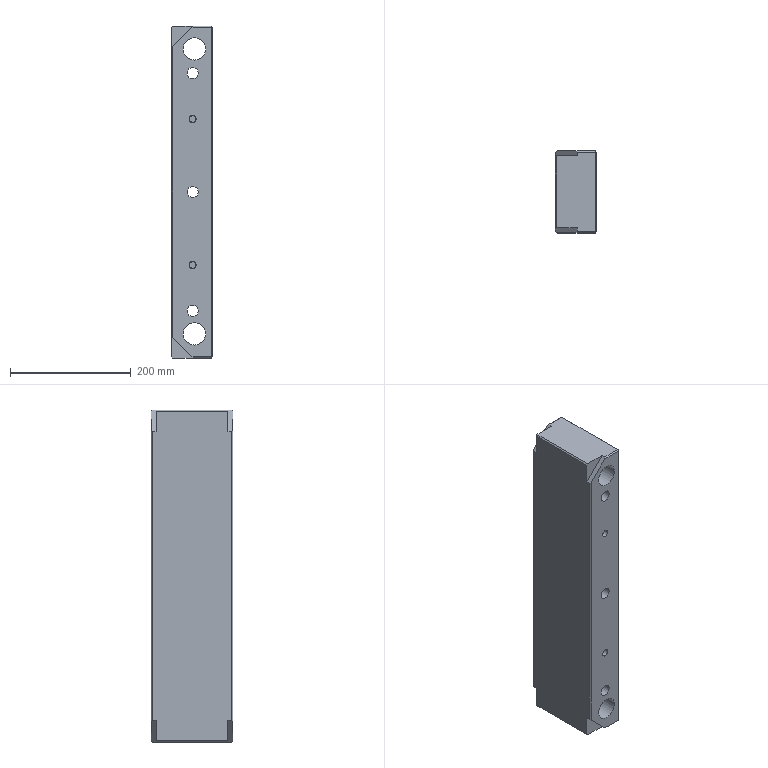Part | STEP file | SPACE-PLATE_id498_x_t | 1 solid | 62 faces | box 68 x 135 x 550 mm | volume 4420744 mm3 | plane 42 | cylinder 16 | other 2 | cone 2 | commonest cylinder face diameters 10 x9 18.5 x3 12 x2 37 x2